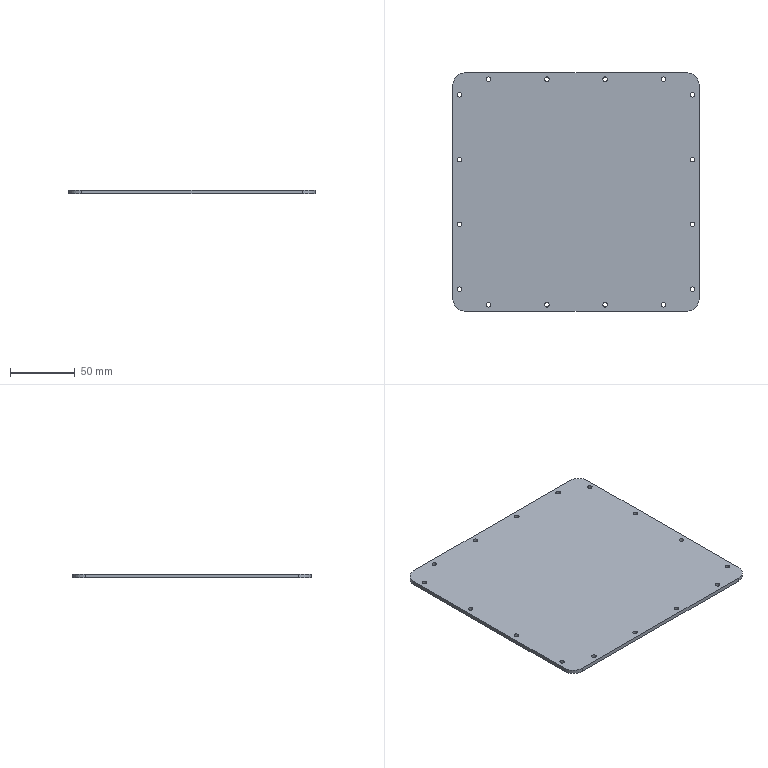Part | STEP file | GLSJ-10-49 | 1 solid | 42 faces | box 190 x 184 x 3 mm | volume 104161 mm3 | cylinder 36 | plane 6 | commonest cylinder face diameters 3.5 x32 20 x4